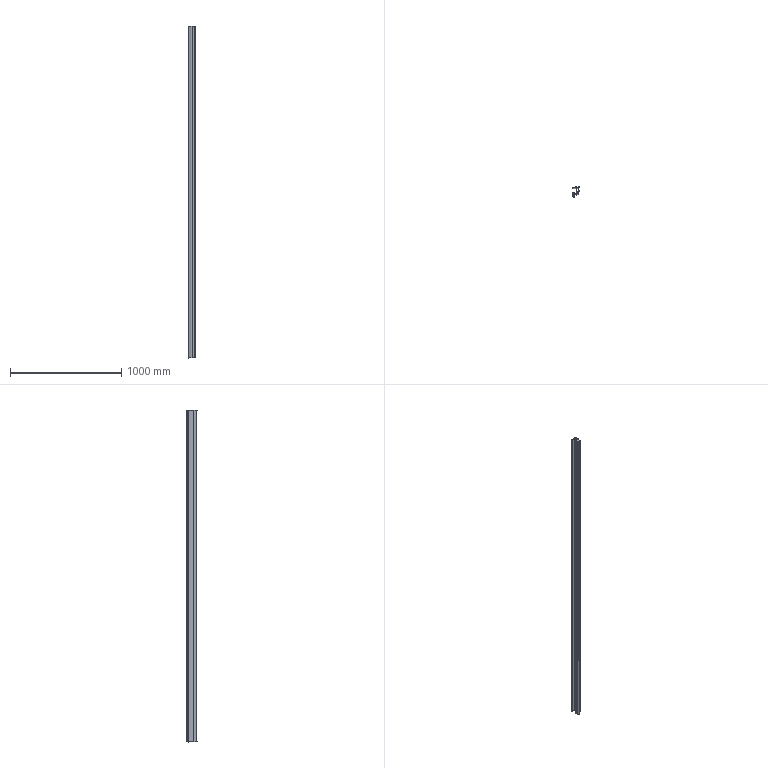Part | STEP file | 51E-01143JG10 | 1 solid | 154 faces | box 62 x 90 x 2980 mm | volume 2562098 mm3 | plane 81 | cylinder 73 | commonest cylinder face diameters 1 x40 0.4 x7 4 x6 6 x5 2 x4 9 x4